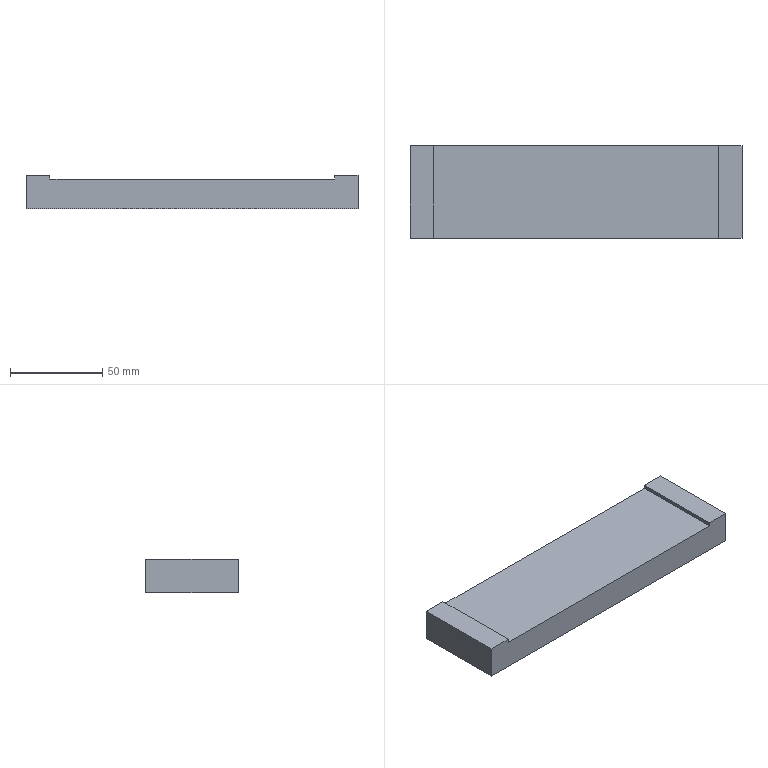Part | STEP file | 001-008-Traverse module gripper mounting plate | 1 solid | 10 faces | box 180 x 50 x 18 mm | volume 146550 mm3 | plane 10
STEP:
#1=CARTESIAN_POINT('',(0.,0.,0.));
#2=DIRECTION('',(0.,0.,1.));
#3=DIRECTION('',(1.,0.,0.));
#4=AXIS2_PLACEMENT_3D('',#1,#2,#3);
#5=CARTESIAN_POINT('',(-90.,-25.,18.));
#6=VERTEX_POINT('',#5);
#7=CARTESIAN_POINT('',(-77.,-25.,18.));
#8=VERTEX_POINT('',#7);
#9=CARTESIAN_POINT('',(-90.,-25.,18.));
#10=DIRECTION('',(1.,0.,0.));
#11=VECTOR('',#10,1.);
#12=LINE('',#9,#11);
#13=CARTESIAN_POINT('',(0.,0.,18.));
#14=DIRECTION('',(0.,0.,-1.));
#15=DIRECTION('',(-1.,0.,0.));
#16=AXIS2_PLACEMENT_3D('',#13,#14,#15);
#17=PLANE('',#16);
#18=CARTESIAN_POINT('',(90.,-25.));
#19=DIRECTION('',(-1.,0.));
#20=VECTOR('',#19,1.);
#21=LINE('',#18,#20);
#22=(GEOMETRIC_REPRESENTATION_CONTEXT(2)PARAMETRIC_REPRESENTATION_CONTEXT()REPRESENTATION_CONTEXT('',''));
#23=DEFINITIONAL_REPRESENTATION('',(#21),#22);
#24=PCURVE('',#17,#23);
#25=CARTESIAN_POINT('',(-90.,-25.,18.));
#26=DIRECTION('',(0.,1.,0.));
#27=DIRECTION('',(-1.,0.,0.));
#28=AXIS2_PLACEMENT_3D('',#25,#26,#27);
#29=PLANE('',#28);
#30=CARTESIAN_POINT('',(0.,0.));
#31=DIRECTION('',(-1.,0.));
#32=VECTOR('',#31,1.);
#33=LINE('',#30,#32);
#34=(GEOMETRIC_REPRESENTATION_CONTEXT(2)PARAMETRIC_REPRESENTATION_CONTEXT()REPRESENTATION_CONTEXT('',''));
#35=DEFINITIONAL_REPRESENTATION('',(#33),#34);
#36=PCURVE('',#29,#35);
#37=SURFACE_CURVE('',#12,(#24,#36),.PCURVE_S1.);
#38=EDGE_CURVE('',#6,#8,#37,.T.);
#39=ORIENTED_EDGE('',*,*,#38,.T.);
#40=CARTESIAN_POINT('',(-77.,25.,18.));
#41=VERTEX_POINT('',#40);
#42=CARTESIAN_POINT('',(-77.,25.,18.));
#43=DIRECTION('',(0.,-1.,0.));
#44=VECTOR('',#43,1.);
#45=LINE('',#42,#44);
#46=CARTESIAN_POINT('',(77.,25.));
#47=DIRECTION('',(0.,-1.));
#48=VECTOR('',#47,1.);
#49=LINE('',#46,#48);
#50=(GEOMETRIC_REPRESENTATION_CONTEXT(2)PARAMETRIC_REPRESENTATION_CONTEXT()REPRESENTATION_CONTEXT('',''));
#51=DEFINITIONAL_REPRESENTATION('',(#49),#50);
#52=PCURVE('',#17,#51);
#53=CARTESIAN_POINT('',(-77.,25.,18.));
#54=DIRECTION('',(-1.,0.,0.));
#55=DIRECTION('',(0.,-1.,0.));
#56=AXIS2_PLACEMENT_3D('',#53,#54,#55);
#57=PLANE('',#56);
#58=CARTESIAN_POINT('',(0.,0.));
#59=DIRECTION('',(1.,0.));
#60=VECTOR('',#59,1.);
#61=LINE('',#58,#60);
#62=(GEOMETRIC_REPRESENTATION_CONTEXT(2)PARAMETRIC_REPRESENTATION_CONTEXT()REPRESENTATION_CONTEXT('',''));
#63=DEFINITIONAL_REPRESENTATION('',(#61),#62);
#64=PCURVE('',#57,#63);
#65=SURFACE_CURVE('',#45,(#52,#64),.PCURVE_S1.);
#66=EDGE_CURVE('',#41,#8,#65,.T.);
#67=ORIENTED_EDGE('',*,*,#66,.F.);
#68=CARTESIAN_POINT('',(-90.,25.,18.));
#69=VERTEX_POINT('',#68);
#70=CARTESIAN_POINT('',(-90.,25.,18.));
#71=DIRECTION('',(-1.,0.,0.));
#72=VECTOR('',#71,1.);
#73=LINE('',#70,#72);
#74=CARTESIAN_POINT('',(90.,25.));
#75=DIRECTION('',(1.,0.));
#76=VECTOR('',#75,1.);
#77=LINE('',#74,#76);
#78=(GEOMETRIC_REPRESENTATION_CONTEXT(2)PARAMETRIC_REPRESENTATION_CONTEXT()REPRESENTATION_CONTEXT('',''));
#79=DEFINITIONAL_REPRESENTATION('',(#77),#78);
#80=PCURVE('',#17,#79);
#81=CARTESIAN_POINT('',(-90.,25.,18.));
#82=DIRECTION('',(0.,-1.,0.));
#83=DIRECTION('',(1.,0.,0.));
#84=AXIS2_PLACEMENT_3D('',#81,#82,#83);
#85=PLANE('',#84);
#86=CARTESIAN_POINT('',(0.,0.));
#87=DIRECTION('',(-1.,0.));
#88=VECTOR('',#87,1.);
#89=LINE('',#86,#88);
#90=(GEOMETRIC_REPRESENTATION_CONTEXT(2)PARAMETRIC_REPRESENTATION_CONTEXT()REPRESENTATION_CONTEXT('',''));
#91=DEFINITIONAL_REPRESENTATION('',(#89),#90);
#92=PCURVE('',#85,#91);
#93=SURFACE_CURVE('',#73,(#80,#92),.PCURVE_S1.);
#94=EDGE_CURVE('',#41,#69,#93,.T.);
#95=ORIENTED_EDGE('',*,*,#94,.T.);
#96=CARTESIAN_POINT('',(-90.,-25.,18.));
#97=DIRECTION('',(0.,-1.,0.));
#98=VECTOR('',#97,1.);
#99=LINE('',#96,#98);
#100=CARTESIAN_POINT('',(90.,-25.));
#101=DIRECTION('',(0.,-1.));
#102=VECTOR('',#101,1.);
#103=LINE('',#100,#102);
#104=(GEOMETRIC_REPRESENTATION_CONTEXT(2)PARAMETRIC_REPRESENTATION_CONTEXT()REPRESENTATION_CONTEXT('',''));
#105=DEFINITIONAL_REPRESENTATION('',(#103),#104);
#106=PCURVE('',#17,#105);
#107=CARTESIAN_POINT('',(-90.,-25.,18.));
#108=DIRECTION('',(1.,0.,0.));
#109=DIRECTION('',(0.,0.,-1.));
#110=AXIS2_PLACEMENT_3D('',#107,#108,#109);
#111=PLANE('',#110);
#112=CARTESIAN_POINT('',(0.,0.));
#113=DIRECTION('',(0.,-1.));
#114=VECTOR('',#113,1.);
#115=LINE('',#112,#114);
#116=(GEOMETRIC_REPRESENTATION_CONTEXT(2)PARAMETRIC_REPRESENTATION_CONTEXT()REPRESENTATION_CONTEXT('',''));
#117=DEFINITIONAL_REPRESENTATION('',(#115),#116);
#118=PCURVE('',#111,#117);
#119=SURFACE_CURVE('',#99,(#106,#118),.PCURVE_S1.);
#120=EDGE_CURVE('',#69,#6,#119,.T.);
#121=ORIENTED_EDGE('',*,*,#120,.T.);
#122=EDGE_LOOP('',(#39,#67,#95,#121));
#123=FACE_BOUND('',#122,.T.);
#124=ADVANCED_FACE('',(#123),#17,.F.);
#125=CARTESIAN_POINT('',(90.,-25.,0.));
#126=VERTEX_POINT('',#125);
#127=CARTESIAN_POINT('',(90.,25.,0.));
#128=VERTEX_POINT('',#127);
#129=CARTESIAN_POINT('',(90.,-25.,0.));
#130=DIRECTION('',(0.,1.,0.));
#131=VECTOR('',#130,1.);
#132=LINE('',#129,#131);
#133=CARTESIAN_POINT('',(90.,-25.,18.));
#134=DIRECTION('',(-1.,0.,0.));
#135=DIRECTION('',(0.,-1.,0.));
#136=AXIS2_PLACEMENT_3D('',#133,#134,#135);
#137=PLANE('',#136);
#138=CARTESIAN_POINT('',(0.,-18.));
#139=DIRECTION('',(-1.,0.));
#140=VECTOR('',#139,1.);
#141=LINE('',#138,#140);
#142=(GEOMETRIC_REPRESENTATION_CONTEXT(2)PARAMETRIC_REPRESENTATION_CONTEXT()REPRESENTATION_CONTEXT('',''));
#143=DEFINITIONAL_REPRESENTATION('',(#141),#142);
#144=PCURVE('',#137,#143);
#145=CARTESIAN_POINT('',(0.,0.,0.));
#146=DIRECTION('',(0.,0.,-1.));
#147=DIRECTION('',(-1.,0.,0.));
#148=AXIS2_PLACEMENT_3D('',#145,#146,#147);
#149=PLANE('',#148);
#150=CARTESIAN_POINT('',(-90.,-25.));
#151=DIRECTION('',(0.,1.));
#152=VECTOR('',#151,1.);
#153=LINE('',#150,#152);
#154=(GEOMETRIC_REPRESENTATION_CONTEXT(2)PARAMETRIC_REPRESENTATION_CONTEXT()REPRESENTATION_CONTEXT('',''));
#155=DEFINITIONAL_REPRESENTATION('',(#153),#154);
#156=PCURVE('',#149,#155);
#157=SURFACE_CURVE('',#132,(#144,#156),.PCURVE_S1.);
#158=EDGE_CURVE('',#126,#128,#157,.T.);
#159=ORIENTED_EDGE('',*,*,#158,.T.);
#160=CARTESIAN_POINT('',(90.,25.,18.));
#161=VERTEX_POINT('',#160);
#162=CARTESIAN_POINT('',(90.,25.,18.));
#163=DIRECTION('',(0.,0.,-1.));
#164=VECTOR('',#163,1.);
#165=LINE('',#162,#164);
#166=CARTESIAN_POINT('',(-50.,0.));
#167=DIRECTION('',(0.,-1.));
#168=VECTOR('',#167,1.);
#169=LINE('',#166,#168);
#170=(GEOMETRIC_REPRESENTATION_CONTEXT(2)PARAMETRIC_REPRESENTATION_CONTEXT()REPRESENTATION_CONTEXT('',''));
#171=DEFINITIONAL_REPRESENTATION('',(#169),#170);
#172=PCURVE('',#137,#171);
#173=CARTESIAN_POINT('',(180.,0.));
#174=DIRECTION('',(0.,-1.));
#175=VECTOR('',#174,1.);
#176=LINE('',#173,#175);
#177=(GEOMETRIC_REPRESENTATION_CONTEXT(2)PARAMETRIC_REPRESENTATION_CONTEXT()REPRESENTATION_CONTEXT('',''));
#178=DEFINITIONAL_REPRESENTATION('',(#176),#177);
#179=PCURVE('',#85,#178);
#180=SURFACE_CURVE('',#165,(#172,#179),.PCURVE_S1.);
#181=EDGE_CURVE('',#161,#128,#180,.T.);
#182=ORIENTED_EDGE('',*,*,#181,.F.);
#183=CARTESIAN_POINT('',(90.,-25.,18.));
#184=VERTEX_POINT('',#183);
#185=CARTESIAN_POINT('',(90.,-25.,18.));
#186=DIRECTION('',(0.,1.,0.));
#187=VECTOR('',#186,1.);
#188=LINE('',#185,#187);
#189=CARTESIAN_POINT('',(0.,0.));
#190=DIRECTION('',(-1.,0.));
#191=VECTOR('',#190,1.);
#192=LINE('',#189,#191);
#193=(GEOMETRIC_REPRESENTATION_CONTEXT(2)PARAMETRIC_REPRESENTATION_CONTEXT()REPRESENTATION_CONTEXT('',''));
#194=DEFINITIONAL_REPRESENTATION('',(#192),#193);
#195=PCURVE('',#137,#194);
#196=CARTESIAN_POINT('',(0.,0.,18.));
#197=DIRECTION('',(0.,0.,-1.));
#198=DIRECTION('',(-1.,0.,0.));
#199=AXIS2_PLACEMENT_3D('',#196,#197,#198);
#200=PLANE('',#199);
#201=CARTESIAN_POINT('',(-90.,-25.));
#202=DIRECTION('',(0.,1.));
#203=VECTOR('',#202,1.);
#204=LINE('',#201,#203);
#205=(GEOMETRIC_REPRESENTATION_CONTEXT(2)PARAMETRIC_REPRESENTATION_CONTEXT()REPRESENTATION_CONTEXT('',''));
#206=DEFINITIONAL_REPRESENTATION('',(#204),#205);
#207=PCURVE('',#200,#206);
#208=SURFACE_CURVE('',#188,(#195,#207),.PCURVE_S1.);
#209=EDGE_CURVE('',#184,#161,#208,.T.);
#210=ORIENTED_EDGE('',*,*,#209,.F.);
#211=CARTESIAN_POINT('',(90.,-25.,18.));
#212=DIRECTION('',(0.,0.,-1.));
#213=VECTOR('',#212,1.);
#214=LINE('',#211,#213);
#215=CARTESIAN_POINT('',(0.,0.));
#216=DIRECTION('',(0.,-1.));
#217=VECTOR('',#216,1.);
#218=LINE('',#215,#217);
#219=(GEOMETRIC_REPRESENTATION_CONTEXT(2)PARAMETRIC_REPRESENTATION_CONTEXT()REPRESENTATION_CONTEXT('',''));
#220=DEFINITIONAL_REPRESENTATION('',(#218),#219);
#221=PCURVE('',#137,#220);
#222=CARTESIAN_POINT('',(-180.,0.));
#223=DIRECTION('',(0.,-1.));
#224=VECTOR('',#223,1.);
#225=LINE('',#222,#224);
#226=(GEOMETRIC_REPRESENTATION_CONTEXT(2)PARAMETRIC_REPRESENTATION_CONTEXT()REPRESENTATION_CONTEXT('',''));
#227=DEFINITIONAL_REPRESENTATION('',(#225),#226);
#228=PCURVE('',#29,#227);
#229=SURFACE_CURVE('',#214,(#221,#228),.PCURVE_S1.);
#230=EDGE_CURVE('',#184,#126,#229,.T.);
#231=ORIENTED_EDGE('',*,*,#230,.T.);
#232=EDGE_LOOP('',(#159,#182,#210,#231));
#233=FACE_BOUND('',#232,.T.);
#234=ADVANCED_FACE('',(#233),#137,.F.);
#235=ORIENTED_EDGE('',*,*,#94,.F.);
#236=CARTESIAN_POINT('',(-77.,25.,16.));
#237=VERTEX_POINT('',#236);
#238=CARTESIAN_POINT('',(-77.,25.,18.));
#239=DIRECTION('',(0.,0.,-1.));
#240=VECTOR('',#239,1.);
#241=LINE('',#238,#240);
#242=CARTESIAN_POINT('',(13.,0.));
#243=DIRECTION('',(0.,-1.));
#244=VECTOR('',#243,1.);
#245=LINE('',#242,#244);
#246=(GEOMETRIC_REPRESENTATION_CONTEXT(2)PARAMETRIC_REPRESENTATION_CONTEXT()REPRESENTATION_CONTEXT('',''));
#247=DEFINITIONAL_REPRESENTATION('',(#245),#246);
#248=PCURVE('',#85,#247);
#249=CARTESIAN_POINT('',(0.,0.));
#250=DIRECTION('',(0.,-1.));
#251=VECTOR('',#250,1.);
#252=LINE('',#249,#251);
#253=(GEOMETRIC_REPRESENTATION_CONTEXT(2)PARAMETRIC_REPRESENTATION_CONTEXT()REPRESENTATION_CONTEXT('',''));
#254=DEFINITIONAL_REPRESENTATION('',(#252),#253);
#255=PCURVE('',#57,#254);
#256=SURFACE_CURVE('',#241,(#248,#255),.PCURVE_S1.);
#257=EDGE_CURVE('',#41,#237,#256,.T.);
#258=ORIENTED_EDGE('',*,*,#257,.T.);
#259=CARTESIAN_POINT('',(77.5,25.,16.));
#260=VERTEX_POINT('',#259);
#261=CARTESIAN_POINT('',(-77.,25.,16.));
#262=DIRECTION('',(1.,0.,0.));
#263=VECTOR('',#262,1.);
#264=LINE('',#261,#263);
#265=CARTESIAN_POINT('',(13.,-2.));
#266=DIRECTION('',(1.,0.));
#267=VECTOR('',#266,1.);
#268=LINE('',#265,#267);
#269=(GEOMETRIC_REPRESENTATION_CONTEXT(2)PARAMETRIC_REPRESENTATION_CONTEXT()REPRESENTATION_CONTEXT('',''));
#270=DEFINITIONAL_REPRESENTATION('',(#268),#269);
#271=PCURVE('',#85,#270);
#272=CARTESIAN_POINT('',(-77.,25.,16.));
#273=DIRECTION('',(0.,0.,-1.));
#274=DIRECTION('',(-1.,0.,0.));
#275=AXIS2_PLACEMENT_3D('',#272,#273,#274);
#276=PLANE('',#275);
#277=CARTESIAN_POINT('',(0.,0.));
#278=DIRECTION('',(-1.,0.));
#279=VECTOR('',#278,1.);
#280=LINE('',#277,#279);
#281=(GEOMETRIC_REPRESENTATION_CONTEXT(2)PARAMETRIC_REPRESENTATION_CONTEXT()REPRESENTATION_CONTEXT('',''));
#282=DEFINITIONAL_REPRESENTATION('',(#280),#281);
#283=PCURVE('',#276,#282);
#284=SURFACE_CURVE('',#264,(#271,#283),.PCURVE_S1.);
#285=EDGE_CURVE('',#237,#260,#284,.T.);
#286=ORIENTED_EDGE('',*,*,#285,.T.);
#287=CARTESIAN_POINT('',(77.5,25.,18.));
#288=VERTEX_POINT('',#287);
#289=CARTESIAN_POINT('',(77.5,25.,18.));
#290=DIRECTION('',(0.,0.,1.));
#291=VECTOR('',#290,1.);
#292=LINE('',#289,#291);
#293=CARTESIAN_POINT('',(167.5,0.));
#294=DIRECTION('',(0.,1.));
#295=VECTOR('',#294,1.);
#296=LINE('',#293,#295);
#297=(GEOMETRIC_REPRESENTATION_CONTEXT(2)PARAMETRIC_REPRESENTATION_CONTEXT()REPRESENTATION_CONTEXT('',''));
#298=DEFINITIONAL_REPRESENTATION('',(#296),#297);
#299=PCURVE('',#85,#298);
#300=CARTESIAN_POINT('',(77.5,25.,18.));
#301=DIRECTION('',(1.,0.,0.));
#302=DIRECTION('',(0.,1.,0.));
#303=AXIS2_PLACEMENT_3D('',#300,#301,#302);
#304=PLANE('',#303);
#305=CARTESIAN_POINT('',(0.,0.));
#306=DIRECTION('',(0.,1.));
#307=VECTOR('',#306,1.);
#308=LINE('',#305,#307);
#309=(GEOMETRIC_REPRESENTATION_CONTEXT(2)PARAMETRIC_REPRESENTATION_CONTEXT()REPRESENTATION_CONTEXT('',''));
#310=DEFINITIONAL_REPRESENTATION('',(#308),#309);
#311=PCURVE('',#304,#310);
#312=SURFACE_CURVE('',#292,(#299,#311),.PCURVE_S1.);
#313=EDGE_CURVE('',#260,#288,#312,.T.);
#314=ORIENTED_EDGE('',*,*,#313,.T.);
#315=CARTESIAN_POINT('',(-90.,25.,18.));
#316=DIRECTION('',(-1.,0.,0.));
#317=VECTOR('',#316,1.);
#318=LINE('',#315,#317);
#319=CARTESIAN_POINT('',(0.,0.));
#320=DIRECTION('',(-1.,0.));
#321=VECTOR('',#320,1.);
#322=LINE('',#319,#321);
#323=(GEOMETRIC_REPRESENTATION_CONTEXT(2)PARAMETRIC_REPRESENTATION_CONTEXT()REPRESENTATION_CONTEXT('',''));
#324=DEFINITIONAL_REPRESENTATION('',(#322),#323);
#325=PCURVE('',#85,#324);
#326=CARTESIAN_POINT('',(90.,25.));
#327=DIRECTION('',(1.,0.));
#328=VECTOR('',#327,1.);
#329=LINE('',#326,#328);
#330=(GEOMETRIC_REPRESENTATION_CONTEXT(2)PARAMETRIC_REPRESENTATION_CONTEXT()REPRESENTATION_CONTEXT('',''));
#331=DEFINITIONAL_REPRESENTATION('',(#329),#330);
#332=PCURVE('',#200,#331);
#333=SURFACE_CURVE('',#318,(#325,#332),.PCURVE_S1.);
#334=EDGE_CURVE('',#161,#288,#333,.T.);
#335=ORIENTED_EDGE('',*,*,#334,.F.);
#336=ORIENTED_EDGE('',*,*,#181,.T.);
#337=CARTESIAN_POINT('',(-90.,25.,0.));
#338=VERTEX_POINT('',#337);
#339=CARTESIAN_POINT('',(-90.,25.,0.));
#340=DIRECTION('',(-1.,0.,0.));
#341=VECTOR('',#340,1.);
#342=LINE('',#339,#341);
#343=CARTESIAN_POINT('',(0.,-18.));
#344=DIRECTION('',(-1.,0.));
#345=VECTOR('',#344,1.);
#346=LINE('',#343,#345);
#347=(GEOMETRIC_REPRESENTATION_CONTEXT(2)PARAMETRIC_REPRESENTATION_CONTEXT()REPRESENTATION_CONTEXT('',''));
#348=DEFINITIONAL_REPRESENTATION('',(#346),#347);
#349=PCURVE('',#85,#348);
#350=CARTESIAN_POINT('',(90.,25.));
#351=DIRECTION('',(1.,0.));
#352=VECTOR('',#351,1.);
#353=LINE('',#350,#352);
#354=(GEOMETRIC_REPRESENTATION_CONTEXT(2)PARAMETRIC_REPRESENTATION_CONTEXT()REPRESENTATION_CONTEXT('',''));
#355=DEFINITIONAL_REPRESENTATION('',(#353),#354);
#356=PCURVE('',#149,#355);
#357=SURFACE_CURVE('',#342,(#349,#356),.PCURVE_S1.);
#358=EDGE_CURVE('',#128,#338,#357,.T.);
#359=ORIENTED_EDGE('',*,*,#358,.T.);
#360=CARTESIAN_POINT('',(-90.,25.,18.));
#361=DIRECTION('',(0.,0.,-1.));
#362=VECTOR('',#361,1.);
#363=LINE('',#360,#362);
#364=CARTESIAN_POINT('',(0.,0.));
#365=DIRECTION('',(0.,-1.));
#366=VECTOR('',#365,1.);
#367=LINE('',#364,#366);
#368=(GEOMETRIC_REPRESENTATION_CONTEXT(2)PARAMETRIC_REPRESENTATION_CONTEXT()REPRESENTATION_CONTEXT('',''));
#369=DEFINITIONAL_REPRESENTATION('',(#367),#368);
#370=PCURVE('',#85,#369);
#371=CARTESIAN_POINT('',(0.,50.));
#372=DIRECTION('',(1.,0.));
#373=VECTOR('',#372,1.);
#374=LINE('',#371,#373);
#375=(GEOMETRIC_REPRESENTATION_CONTEXT(2)PARAMETRIC_REPRESENTATION_CONTEXT()REPRESENTATION_CONTEXT('',''));
#376=DEFINITIONAL_REPRESENTATION('',(#374),#375);
#377=PCURVE('',#111,#376);
#378=SURFACE_CURVE('',#363,(#370,#377),.PCURVE_S1.);
#379=EDGE_CURVE('',#69,#338,#378,.T.);
#380=ORIENTED_EDGE('',*,*,#379,.F.);
#381=EDGE_LOOP('',(#235,#258,#286,#314,#335,#336,#359,#380));
#382=FACE_BOUND('',#381,.T.);
#383=ADVANCED_FACE('',(#382),#85,.F.);
#384=CARTESIAN_POINT('',(-90.,-25.,0.));
#385=VERTEX_POINT('',#384);
#386=CARTESIAN_POINT('',(-90.,-25.,0.));
#387=DIRECTION('',(0.,-1.,0.));
#388=VECTOR('',#387,1.);
#389=LINE('',#386,#388);
#390=CARTESIAN_POINT('',(18.,0.));
#391=DIRECTION('',(0.,-1.));
#392=VECTOR('',#391,1.);
#393=LINE('',#390,#392);
#394=(GEOMETRIC_REPRESENTATION_CONTEXT(2)PARAMETRIC_REPRESENTATION_CONTEXT()REPRESENTATION_CONTEXT('',''));
#395=DEFINITIONAL_REPRESENTATION('',(#393),#394);
#396=PCURVE('',#111,#395);
#397=CARTESIAN_POINT('',(90.,-25.));
#398=DIRECTION('',(0.,-1.));
#399=VECTOR('',#398,1.);
#400=LINE('',#397,#399);
#401=(GEOMETRIC_REPRESENTATION_CONTEXT(2)PARAMETRIC_REPRESENTATION_CONTEXT()REPRESENTATION_CONTEXT('',''));
#402=DEFINITIONAL_REPRESENTATION('',(#400),#401);
#403=PCURVE('',#149,#402);
#404=SURFACE_CURVE('',#389,(#396,#403),.PCURVE_S1.);
#405=EDGE_CURVE('',#338,#385,#404,.T.);
#406=ORIENTED_EDGE('',*,*,#405,.T.);
#407=CARTESIAN_POINT('',(-90.,-25.,18.));
#408=DIRECTION('',(0.,0.,-1.));
#409=VECTOR('',#408,1.);
#410=LINE('',#407,#409);
#411=CARTESIAN_POINT('',(0.,0.));
#412=DIRECTION('',(1.,0.));
#413=VECTOR('',#412,1.);
#414=LINE('',#411,#413);
#415=(GEOMETRIC_REPRESENTATION_CONTEXT(2)PARAMETRIC_REPRESENTATION_CONTEXT()REPRESENTATION_CONTEXT('',''));
#416=DEFINITIONAL_REPRESENTATION('',(#414),#415);
#417=PCURVE('',#111,#416);
#418=CARTESIAN_POINT('',(0.,0.));
#419=DIRECTION('',(0.,-1.));
#420=VECTOR('',#419,1.);
#421=LINE('',#418,#420);
#422=(GEOMETRIC_REPRESENTATION_CONTEXT(2)PARAMETRIC_REPRESENTATION_CONTEXT()REPRESENTATION_CONTEXT('',''));
#423=DEFINITIONAL_REPRESENTATION('',(#421),#422);
#424=PCURVE('',#29,#423);
#425=SURFACE_CURVE('',#410,(#417,#424),.PCURVE_S1.);
#426=EDGE_CURVE('',#6,#385,#425,.T.);
#427=ORIENTED_EDGE('',*,*,#426,.F.);
#428=ORIENTED_EDGE('',*,*,#120,.F.);
#429=ORIENTED_EDGE('',*,*,#379,.T.);
#430=EDGE_LOOP('',(#406,#427,#428,#429));
#431=FACE_BOUND('',#430,.T.);
#432=ADVANCED_FACE('',(#431),#111,.F.);
#433=CARTESIAN_POINT('',(-77.,-25.,16.));
#434=VERTEX_POINT('',#433);
#435=CARTESIAN_POINT('',(77.5,-25.,16.));
#436=VERTEX_POINT('',#435);
#437=CARTESIAN_POINT('',(-77.,-25.,16.));
#438=DIRECTION('',(1.,0.,0.));
#439=VECTOR('',#438,1.);
#440=LINE('',#437,#439);
#441=CARTESIAN_POINT('',(-13.,-2.));
#442=DIRECTION('',(-1.,0.));
#443=VECTOR('',#442,1.);
#444=LINE('',#441,#443);
#445=(GEOMETRIC_REPRESENTATION_CONTEXT(2)PARAMETRIC_REPRESENTATION_CONTEXT()REPRESENTATION_CONTEXT('',''));
#446=DEFINITIONAL_REPRESENTATION('',(#444),#445);
#447=PCURVE('',#29,#446);
#448=CARTESIAN_POINT('',(0.,-50.));
#449=DIRECTION('',(-1.,0.));
#450=VECTOR('',#449,1.);
#451=LINE('',#448,#450);
#452=(GEOMETRIC_REPRESENTATION_CONTEXT(2)PARAMETRIC_REPRESENTATION_CONTEXT()REPRESENTATION_CONTEXT('',''));
#453=DEFINITIONAL_REPRESENTATION('',(#451),#452);
#454=PCURVE('',#276,#453);
#455=SURFACE_CURVE('',#440,(#447,#454),.PCURVE_S1.);
#456=EDGE_CURVE('',#434,#436,#455,.T.);
#457=ORIENTED_EDGE('',*,*,#456,.F.);
#458=CARTESIAN_POINT('',(-77.,-25.,18.));
#459=DIRECTION('',(0.,0.,-1.));
#460=VECTOR('',#459,1.);
#461=LINE('',#458,#460);
#462=CARTESIAN_POINT('',(-13.,0.));
#463=DIRECTION('',(0.,-1.));
#464=VECTOR('',#463,1.);
#465=LINE('',#462,#464);
#466=(GEOMETRIC_REPRESENTATION_CONTEXT(2)PARAMETRIC_REPRESENTATION_CONTEXT()REPRESENTATION_CONTEXT('',''));
#467=DEFINITIONAL_REPRESENTATION('',(#465),#466);
#468=PCURVE('',#29,#467);
#469=CARTESIAN_POINT('',(50.,0.));
#470=DIRECTION('',(0.,-1.));
#471=VECTOR('',#470,1.);
#472=LINE('',#469,#471);
#473=(GEOMETRIC_REPRESENTATION_CONTEXT(2)PARAMETRIC_REPRESENTATION_CONTEXT()REPRESENTATION_CONTEXT('',''));
#474=DEFINITIONAL_REPRESENTATION('',(#472),#473);
#475=PCURVE('',#57,#474);
#476=SURFACE_CURVE('',#461,(#468,#475),.PCURVE_S1.);
#477=EDGE_CURVE('',#8,#434,#476,.T.);
#478=ORIENTED_EDGE('',*,*,#477,.F.);
#479=ORIENTED_EDGE('',*,*,#38,.F.);
#480=ORIENTED_EDGE('',*,*,#426,.T.);
#481=CARTESIAN_POINT('',(-90.,-25.,0.));
#482=DIRECTION('',(1.,0.,0.));
#483=VECTOR('',#482,1.);
#484=LINE('',#481,#483);
#485=CARTESIAN_POINT('',(0.,-18.));
#486=DIRECTION('',(-1.,0.));
#487=VECTOR('',#486,1.);
#488=LINE('',#485,#487);
#489=(GEOMETRIC_REPRESENTATION_CONTEXT(2)PARAMETRIC_REPRESENTATION_CONTEXT()REPRESENTATION_CONTEXT('',''));
#490=DEFINITIONAL_REPRESENTATION('',(#488),#489);
#491=PCURVE('',#29,#490);
#492=CARTESIAN_POINT('',(90.,-25.));
#493=DIRECTION('',(-1.,0.));
#494=VECTOR('',#493,1.);
#495=LINE('',#492,#494);
#496=(GEOMETRIC_REPRESENTATION_CONTEXT(2)PARAMETRIC_REPRESENTATION_CONTEXT()REPRESENTATION_CONTEXT('',''));
#497=DEFINITIONAL_REPRESENTATION('',(#495),#496);
#498=PCURVE('',#149,#497);
#499=SURFACE_CURVE('',#484,(#491,#498),.PCURVE_S1.);
#500=EDGE_CURVE('',#385,#126,#499,.T.);
#501=ORIENTED_EDGE('',*,*,#500,.T.);
#502=ORIENTED_EDGE('',*,*,#230,.F.);
#503=CARTESIAN_POINT('',(77.5,-25.,18.));
#504=VERTEX_POINT('',#503);
#505=CARTESIAN_POINT('',(-90.,-25.,18.));
#506=DIRECTION('',(1.,0.,0.));
#507=VECTOR('',#506,1.);
#508=LINE('',#505,#507);
#509=CARTESIAN_POINT('',(0.,0.));
#510=DIRECTION('',(-1.,0.));
#511=VECTOR('',#510,1.);
#512=LINE('',#509,#511);
#513=(GEOMETRIC_REPRESENTATION_CONTEXT(2)PARAMETRIC_REPRESENTATION_CONTEXT()REPRESENTATION_CONTEXT('',''));
#514=DEFINITIONAL_REPRESENTATION('',(#512),#513);
#515=PCURVE('',#29,#514);
#516=CARTESIAN_POINT('',(90.,-25.));
#517=DIRECTION('',(-1.,0.));
#518=VECTOR('',#517,1.);
#519=LINE('',#516,#518);
#520=(GEOMETRIC_REPRESENTATION_CONTEXT(2)PARAMETRIC_REPRESENTATION_CONTEXT()REPRESENTATION_CONTEXT('',''));
#521=DEFINITIONAL_REPRESENTATION('',(#519),#520);
#522=PCURVE('',#200,#521);
#523=SURFACE_CURVE('',#508,(#515,#522),.PCURVE_S1.);
#524=EDGE_CURVE('',#504,#184,#523,.T.);
#525=ORIENTED_EDGE('',*,*,#524,.F.);
#526=CARTESIAN_POINT('',(77.5,-25.,18.));
#527=DIRECTION('',(0.,0.,1.));
#528=VECTOR('',#527,1.);
#529=LINE('',#526,#528);
#530=CARTESIAN_POINT('',(-167.5,0.));
#531=DIRECTION('',(0.,1.));
#532=VECTOR('',#531,1.);
#533=LINE('',#530,#532);
#534=(GEOMETRIC_REPRESENTATION_CONTEXT(2)PARAMETRIC_REPRESENTATION_CONTEXT()REPRESENTATION_CONTEXT('',''));
#535=DEFINITIONAL_REPRESENTATION('',(#533),#534);
#536=PCURVE('',#29,#535);
#537=CARTESIAN_POINT('',(-50.,0.));
#538=DIRECTION('',(0.,1.));
#539=VECTOR('',#538,1.);
#540=LINE('',#537,#539);
#541=(GEOMETRIC_REPRESENTATION_CONTEXT(2)PARAMETRIC_REPRESENTATION_CONTEXT()REPRESENTATION_CONTEXT('',''));
#542=DEFINITIONAL_REPRESENTATION('',(#540),#541);
#543=PCURVE('',#304,#542);
#544=SURFACE_CURVE('',#529,(#536,#543),.PCURVE_S1.);
#545=EDGE_CURVE('',#436,#504,#544,.T.);
#546=ORIENTED_EDGE('',*,*,#545,.F.);
#547=EDGE_LOOP('',(#457,#478,#479,#480,#501,#502,#525,#546));
#548=FACE_BOUND('',#547,.T.);
#549=ADVANCED_FACE('',(#548),#29,.F.);
#550=ORIENTED_EDGE('',*,*,#334,.T.);
#551=CARTESIAN_POINT('',(77.5,25.,18.));
#552=DIRECTION('',(0.,-1.,0.));
#553=VECTOR('',#552,1.);
#554=LINE('',#551,#553);
#555=CARTESIAN_POINT('',(-77.5,25.));
#556=DIRECTION('',(0.,-1.));
#557=VECTOR('',#556,1.);
#558=LINE('',#555,#557);
#559=(GEOMETRIC_REPRESENTATION_CONTEXT(2)PARAMETRIC_REPRESENTATION_CONTEXT()REPRESENTATION_CONTEXT('',''));
#560=DEFINITIONAL_REPRESENTATION('',(#558),#559);
#561=PCURVE('',#200,#560);
#562=CARTESIAN_POINT('',(0.,0.));
#563=DIRECTION('',(-1.,0.));
#564=VECTOR('',#563,1.);
#565=LINE('',#562,#564);
#566=(GEOMETRIC_REPRESENTATION_CONTEXT(2)PARAMETRIC_REPRESENTATION_CONTEXT()REPRESENTATION_CONTEXT('',''));
#567=DEFINITIONAL_REPRESENTATION('',(#565),#566);
#568=PCURVE('',#304,#567);
#569=SURFACE_CURVE('',#554,(#561,#568),.PCURVE_S1.);
#570=EDGE_CURVE('',#288,#504,#569,.T.);
#571=ORIENTED_EDGE('',*,*,#570,.T.);
#572=ORIENTED_EDGE('',*,*,#524,.T.);
#573=ORIENTED_EDGE('',*,*,#209,.T.);
#574=EDGE_LOOP('',(#550,#571,#572,#573));
#575=FACE_BOUND('',#574,.T.);
#576=ADVANCED_FACE('',(#575),#200,.F.);
#577=ORIENTED_EDGE('',*,*,#158,.F.);
#578=ORIENTED_EDGE('',*,*,#500,.F.);
#579=ORIENTED_EDGE('',*,*,#405,.F.);
#580=ORIENTED_EDGE('',*,*,#358,.F.);
#581=EDGE_LOOP('',(#577,#578,#579,#580));
#582=FACE_BOUND('',#581,.T.);
#583=ADVANCED_FACE('',(#582),#149,.T.);
#584=ORIENTED_EDGE('',*,*,#477,.T.);
#585=CARTESIAN_POINT('',(-77.,25.,16.));
#586=DIRECTION('',(0.,-1.,0.));
#587=VECTOR('',#586,1.);
#588=LINE('',#585,#587);
#589=CARTESIAN_POINT('',(0.,-2.));
#590=DIRECTION('',(1.,0.));
#591=VECTOR('',#590,1.);
#592=LINE('',#589,#591);
#593=(GEOMETRIC_REPRESENTATION_CONTEXT(2)PARAMETRIC_REPRESENTATION_CONTEXT()REPRESENTATION_CONTEXT('',''));
#594=DEFINITIONAL_REPRESENTATION('',(#592),#593);
#595=PCURVE('',#57,#594);
#596=CARTESIAN_POINT('',(0.,0.));
#597=DIRECTION('',(0.,-1.));
#598=VECTOR('',#597,1.);
#599=LINE('',#596,#598);
#600=(GEOMETRIC_REPRESENTATION_CONTEXT(2)PARAMETRIC_REPRESENTATION_CONTEXT()REPRESENTATION_CONTEXT('',''));
#601=DEFINITIONAL_REPRESENTATION('',(#599),#600);
#602=PCURVE('',#276,#601);
#603=SURFACE_CURVE('',#588,(#595,#602),.PCURVE_S1.);
#604=EDGE_CURVE('',#237,#434,#603,.T.);
#605=ORIENTED_EDGE('',*,*,#604,.F.);
#606=ORIENTED_EDGE('',*,*,#257,.F.);
#607=ORIENTED_EDGE('',*,*,#66,.T.);
#608=EDGE_LOOP('',(#584,#605,#606,#607));
#609=FACE_BOUND('',#608,.T.);
#610=ADVANCED_FACE('',(#609),#57,.F.);
#611=ORIENTED_EDGE('',*,*,#545,.T.);
#612=ORIENTED_EDGE('',*,*,#570,.F.);
#613=ORIENTED_EDGE('',*,*,#313,.F.);
#614=CARTESIAN_POINT('',(77.5,25.,16.));
#615=DIRECTION('',(0.,-1.,0.));
#616=VECTOR('',#615,1.);
#617=LINE('',#614,#616);
#618=CARTESIAN_POINT('',(0.,-2.));
#619=DIRECTION('',(-1.,0.));
#620=VECTOR('',#619,1.);
#621=LINE('',#618,#620);
#622=(GEOMETRIC_REPRESENTATION_CONTEXT(2)PARAMETRIC_REPRESENTATION_CONTEXT()REPRESENTATION_CONTEXT('',''));
#623=DEFINITIONAL_REPRESENTATION('',(#621),#622);
#624=PCURVE('',#304,#623);
#625=CARTESIAN_POINT('',(-154.5,0.));
#626=DIRECTION('',(0.,-1.));
#627=VECTOR('',#626,1.);
#628=LINE('',#625,#627);
#629=(GEOMETRIC_REPRESENTATION_CONTEXT(2)PARAMETRIC_REPRESENTATION_CONTEXT()REPRESENTATION_CONTEXT('',''));
#630=DEFINITIONAL_REPRESENTATION('',(#628),#629);
#631=PCURVE('',#276,#630);
#632=SURFACE_CURVE('',#617,(#624,#631),.PCURVE_S1.);
#633=EDGE_CURVE('',#260,#436,#632,.T.);
#634=ORIENTED_EDGE('',*,*,#633,.T.);
#635=EDGE_LOOP('',(#611,#612,#613,#634));
#636=FACE_BOUND('',#635,.T.);
#637=ADVANCED_FACE('',(#636),#304,.F.);
#638=ORIENTED_EDGE('',*,*,#456,.T.);
#639=ORIENTED_EDGE('',*,*,#633,.F.);
#640=ORIENTED_EDGE('',*,*,#285,.F.);
#641=ORIENTED_EDGE('',*,*,#604,.T.);
#642=EDGE_LOOP('',(#638,#639,#640,#641));
#643=FACE_BOUND('',#642,.T.);
#644=ADVANCED_FACE('',(#643),#276,.F.);
#645=CLOSED_SHELL('',(#124,#234,#383,#432,#549,#576,#583,#610,#637,#644));
#646=MANIFOLD_SOLID_BREP('',#645);
#647=(LENGTH_UNIT()NAMED_UNIT(*)SI_UNIT(.MILLI.,.METRE.));
#648=UNCERTAINTY_MEASURE_WITH_UNIT(LENGTH_MEASURE(0.0000001),#647,'','');
#649=(NAMED_UNIT(*)PLANE_ANGLE_UNIT()SI_UNIT($,.RADIAN.));
#650=(NAMED_UNIT(*)SI_UNIT($,.STERADIAN.)SOLID_ANGLE_UNIT());
#651=(GEOMETRIC_REPRESENTATION_CONTEXT(3)GLOBAL_UNCERTAINTY_ASSIGNED_CONTEXT((#648))GLOBAL_UNIT_ASSIGNED_CONTEXT((#647,#649,#650))REPRESENTATION_CONTEXT('',''));
#652=ADVANCED_BREP_SHAPE_REPRESENTATION('',(#4,#646),#651);